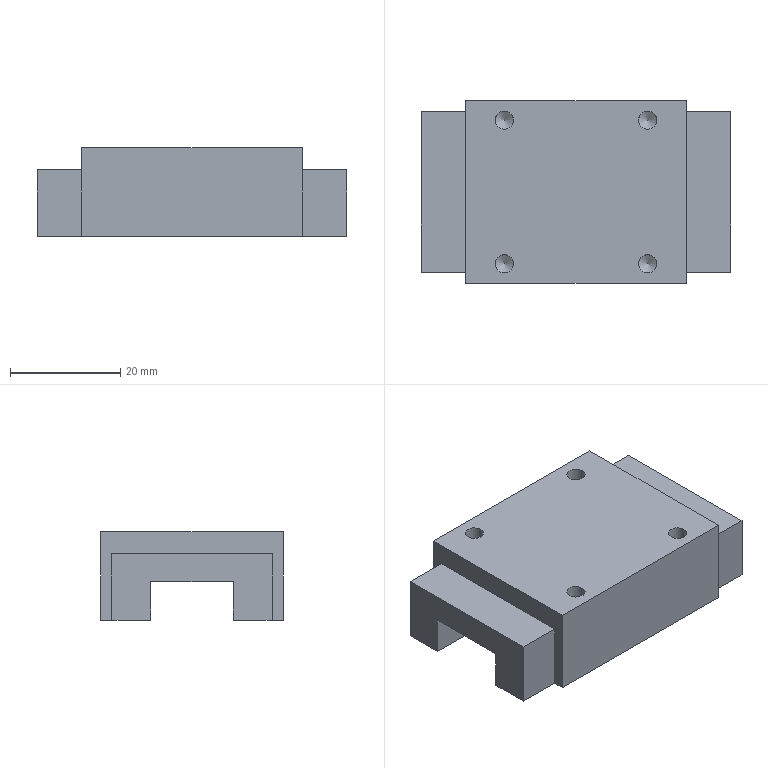Part | STEP file | 1 solid | 26 faces | box 56 x 33 x 16 mm | volume 20352 mm3 | plane 18 | cylinder 4 | cone 4 | commonest cylinder face diameters 3.3 x4